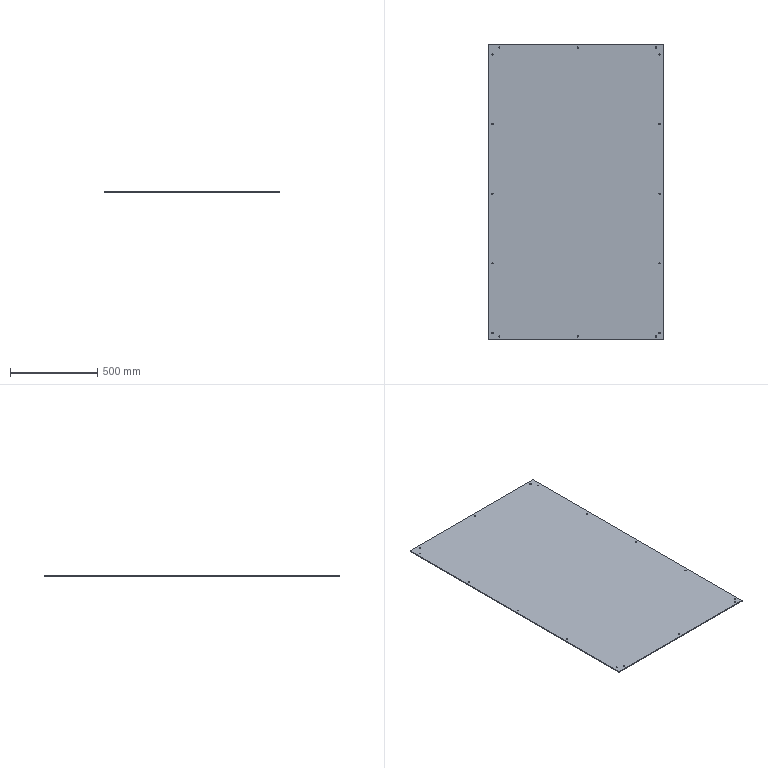Part | STEP file | 平铺封Plate_LE0314013532 | 1 solid | 42 faces | box 1000 x 1700 x 5 mm | volume 8497328 mm3 | cylinder 36 | plane 6 | commonest cylinder face diameters 6.5 x32 4 x4
STEP:
#1=CARTESIAN_POINT('',(463.25,-830.,-2.5));
#2=VERTEX_POINT('',#1);
#3=CARTESIAN_POINT('',(456.75,-830.,-2.5));
#4=VERTEX_POINT('',#3);
#5=CARTESIAN_POINT('',(460.,-830.,-2.5));
#6=DIRECTION('',(0.,0.,-1.));
#7=DIRECTION('',(1.,0.,0.));
#8=AXIS2_PLACEMENT_3D('',#5,#6,#7);
#9=CIRCLE('',#8,3.25);
#10=EDGE_CURVE('',#2,#4,#9,.T.);
#11=ORIENTED_EDGE('',*,*,#10,.T.);
#12=CARTESIAN_POINT('',(456.75,-830.,2.5));
#13=VERTEX_POINT('',#12);
#14=CARTESIAN_POINT('',(456.75,-830.,2.5));
#15=DIRECTION('',(0.,0.,1.));
#16=VECTOR('',#15,1000.);
#17=LINE('',#14,#16);
#18=EDGE_CURVE('',#4,#13,#17,.T.);
#19=ORIENTED_EDGE('',*,*,#18,.T.);
#20=CARTESIAN_POINT('',(463.25,-830.,2.5));
#21=VERTEX_POINT('',#20);
#22=CARTESIAN_POINT('',(460.,-830.,2.5));
#23=DIRECTION('',(0.,0.,-1.));
#24=DIRECTION('',(1.,0.,0.));
#25=AXIS2_PLACEMENT_3D('',#22,#23,#24);
#26=CIRCLE('',#25,3.25);
#27=EDGE_CURVE('',#21,#13,#26,.T.);
#28=ORIENTED_EDGE('',*,*,#27,.F.);
#29=CARTESIAN_POINT('',(463.25,-830.,2.5));
#30=DIRECTION('',(0.,0.,1.));
#31=VECTOR('',#30,1000.);
#32=LINE('',#29,#31);
#33=EDGE_CURVE('',#2,#21,#32,.T.);
#34=ORIENTED_EDGE('',*,*,#33,.F.);
#35=EDGE_LOOP('',(#11,#19,#28,#34));
#36=FACE_OUTER_BOUND('',#35,.T.);
#37=CARTESIAN_POINT('',(460.,-830.,2.5));
#38=DIRECTION('',(0.,0.,1.));
#39=DIRECTION('',(1.,0.,0.));
#40=AXIS2_PLACEMENT_3D('',#37,#38,#39);
#41=CYLINDRICAL_SURFACE('',#40,3.25);
#42=ADVANCED_FACE('',(#36),#41,.F.);
#43=CARTESIAN_POINT('',(463.25,830.,-2.5));
#44=VERTEX_POINT('',#43);
#45=CARTESIAN_POINT('',(456.75,830.,-2.5));
#46=VERTEX_POINT('',#45);
#47=CARTESIAN_POINT('',(460.,830.,-2.5));
#48=DIRECTION('',(0.,0.,-1.));
#49=DIRECTION('',(1.,0.,0.));
#50=AXIS2_PLACEMENT_3D('',#47,#48,#49);
#51=CIRCLE('',#50,3.25);
#52=EDGE_CURVE('',#44,#46,#51,.T.);
#53=ORIENTED_EDGE('',*,*,#52,.T.);
#54=CARTESIAN_POINT('',(456.75,830.,2.5));
#55=VERTEX_POINT('',#54);
#56=CARTESIAN_POINT('',(456.75,830.,2.5));
#57=DIRECTION('',(0.,0.,1.));
#58=VECTOR('',#57,1000.);
#59=LINE('',#56,#58);
#60=EDGE_CURVE('',#46,#55,#59,.T.);
#61=ORIENTED_EDGE('',*,*,#60,.T.);
#62=CARTESIAN_POINT('',(463.25,830.,2.5));
#63=VERTEX_POINT('',#62);
#64=CARTESIAN_POINT('',(460.,830.,2.5));
#65=DIRECTION('',(0.,0.,-1.));
#66=DIRECTION('',(1.,0.,0.));
#67=AXIS2_PLACEMENT_3D('',#64,#65,#66);
#68=CIRCLE('',#67,3.25);
#69=EDGE_CURVE('',#63,#55,#68,.T.);
#70=ORIENTED_EDGE('',*,*,#69,.F.);
#71=CARTESIAN_POINT('',(463.25,830.,2.5));
#72=DIRECTION('',(0.,0.,1.));
#73=VECTOR('',#72,1000.);
#74=LINE('',#71,#73);
#75=EDGE_CURVE('',#44,#63,#74,.T.);
#76=ORIENTED_EDGE('',*,*,#75,.F.);
#77=EDGE_LOOP('',(#53,#61,#70,#76));
#78=FACE_OUTER_BOUND('',#77,.T.);
#79=CARTESIAN_POINT('',(460.,830.,2.5));
#80=DIRECTION('',(0.,0.,1.));
#81=DIRECTION('',(1.,0.,0.));
#82=AXIS2_PLACEMENT_3D('',#79,#80,#81);
#83=CYLINDRICAL_SURFACE('',#82,3.25);
#84=ADVANCED_FACE('',(#78),#83,.F.);
#85=CARTESIAN_POINT('',(-476.75,-810.,-2.5));
#86=VERTEX_POINT('',#85);
#87=CARTESIAN_POINT('',(-483.25,-810.,-2.5));
#88=VERTEX_POINT('',#87);
#89=CARTESIAN_POINT('',(-480.,-810.,-2.5));
#90=DIRECTION('',(0.,0.,-1.));
#91=DIRECTION('',(1.,0.,0.));
#92=AXIS2_PLACEMENT_3D('',#89,#90,#91);
#93=CIRCLE('',#92,3.25);
#94=EDGE_CURVE('',#86,#88,#93,.T.);
#95=ORIENTED_EDGE('',*,*,#94,.T.);
#96=CARTESIAN_POINT('',(-483.25,-810.,2.5));
#97=VERTEX_POINT('',#96);
#98=CARTESIAN_POINT('',(-483.25,-810.,2.5));
#99=DIRECTION('',(0.,0.,1.));
#100=VECTOR('',#99,1000.);
#101=LINE('',#98,#100);
#102=EDGE_CURVE('',#88,#97,#101,.T.);
#103=ORIENTED_EDGE('',*,*,#102,.T.);
#104=CARTESIAN_POINT('',(-476.75,-810.,2.5));
#105=VERTEX_POINT('',#104);
#106=CARTESIAN_POINT('',(-480.,-810.,2.5));
#107=DIRECTION('',(0.,0.,-1.));
#108=DIRECTION('',(1.,0.,0.));
#109=AXIS2_PLACEMENT_3D('',#106,#107,#108);
#110=CIRCLE('',#109,3.25);
#111=EDGE_CURVE('',#105,#97,#110,.T.);
#112=ORIENTED_EDGE('',*,*,#111,.F.);
#113=CARTESIAN_POINT('',(-476.75,-810.,2.5));
#114=DIRECTION('',(0.,0.,1.));
#115=VECTOR('',#114,1000.);
#116=LINE('',#113,#115);
#117=EDGE_CURVE('',#86,#105,#116,.T.);
#118=ORIENTED_EDGE('',*,*,#117,.F.);
#119=EDGE_LOOP('',(#95,#103,#112,#118));
#120=FACE_OUTER_BOUND('',#119,.T.);
#121=CARTESIAN_POINT('',(-480.,-810.,2.5));
#122=DIRECTION('',(0.,0.,1.));
#123=DIRECTION('',(1.,0.,0.));
#124=AXIS2_PLACEMENT_3D('',#121,#122,#123);
#125=CYLINDRICAL_SURFACE('',#124,3.25);
#126=ADVANCED_FACE('',(#120),#125,.F.);
#127=CARTESIAN_POINT('',(-476.75,-410.,-2.5));
#128=VERTEX_POINT('',#127);
#129=CARTESIAN_POINT('',(-483.25,-410.,-2.5));
#130=VERTEX_POINT('',#129);
#131=CARTESIAN_POINT('',(-480.,-410.,-2.5));
#132=DIRECTION('',(0.,0.,-1.));
#133=DIRECTION('',(1.,0.,0.));
#134=AXIS2_PLACEMENT_3D('',#131,#132,#133);
#135=CIRCLE('',#134,3.25);
#136=EDGE_CURVE('',#128,#130,#135,.T.);
#137=ORIENTED_EDGE('',*,*,#136,.T.);
#138=CARTESIAN_POINT('',(-483.25,-410.,2.5));
#139=VERTEX_POINT('',#138);
#140=CARTESIAN_POINT('',(-483.25,-410.,2.5));
#141=DIRECTION('',(0.,0.,1.));
#142=VECTOR('',#141,1000.);
#143=LINE('',#140,#142);
#144=EDGE_CURVE('',#130,#139,#143,.T.);
#145=ORIENTED_EDGE('',*,*,#144,.T.);
#146=CARTESIAN_POINT('',(-476.75,-410.,2.5));
#147=VERTEX_POINT('',#146);
#148=CARTESIAN_POINT('',(-480.,-410.,2.5));
#149=DIRECTION('',(0.,0.,-1.));
#150=DIRECTION('',(1.,0.,0.));
#151=AXIS2_PLACEMENT_3D('',#148,#149,#150);
#152=CIRCLE('',#151,3.25);
#153=EDGE_CURVE('',#147,#139,#152,.T.);
#154=ORIENTED_EDGE('',*,*,#153,.F.);
#155=CARTESIAN_POINT('',(-476.75,-410.,2.5));
#156=DIRECTION('',(0.,0.,1.));
#157=VECTOR('',#156,1000.);
#158=LINE('',#155,#157);
#159=EDGE_CURVE('',#128,#147,#158,.T.);
#160=ORIENTED_EDGE('',*,*,#159,.F.);
#161=EDGE_LOOP('',(#137,#145,#154,#160));
#162=FACE_OUTER_BOUND('',#161,.T.);
#163=CARTESIAN_POINT('',(-480.,-410.,2.5));
#164=DIRECTION('',(0.,0.,1.));
#165=DIRECTION('',(1.,0.,0.));
#166=AXIS2_PLACEMENT_3D('',#163,#164,#165);
#167=CYLINDRICAL_SURFACE('',#166,3.25);
#168=ADVANCED_FACE('',(#162),#167,.F.);
#169=CARTESIAN_POINT('',(-476.75,-10.,-2.5));
#170=VERTEX_POINT('',#169);
#171=CARTESIAN_POINT('',(-483.25,-10.,-2.5));
#172=VERTEX_POINT('',#171);
#173=CARTESIAN_POINT('',(-480.,-10.,-2.5));
#174=DIRECTION('',(0.,0.,-1.));
#175=DIRECTION('',(1.,0.,0.));
#176=AXIS2_PLACEMENT_3D('',#173,#174,#175);
#177=CIRCLE('',#176,3.25);
#178=EDGE_CURVE('',#170,#172,#177,.T.);
#179=ORIENTED_EDGE('',*,*,#178,.T.);
#180=CARTESIAN_POINT('',(-483.25,-10.,2.5));
#181=VERTEX_POINT('',#180);
#182=CARTESIAN_POINT('',(-483.25,-10.,2.5));
#183=DIRECTION('',(0.,0.,1.));
#184=VECTOR('',#183,1000.);
#185=LINE('',#182,#184);
#186=EDGE_CURVE('',#172,#181,#185,.T.);
#187=ORIENTED_EDGE('',*,*,#186,.T.);
#188=CARTESIAN_POINT('',(-476.75,-10.,2.5));
#189=VERTEX_POINT('',#188);
#190=CARTESIAN_POINT('',(-480.,-10.,2.5));
#191=DIRECTION('',(0.,0.,-1.));
#192=DIRECTION('',(1.,0.,0.));
#193=AXIS2_PLACEMENT_3D('',#190,#191,#192);
#194=CIRCLE('',#193,3.25);
#195=EDGE_CURVE('',#189,#181,#194,.T.);
#196=ORIENTED_EDGE('',*,*,#195,.F.);
#197=CARTESIAN_POINT('',(-476.75,-10.,2.5));
#198=DIRECTION('',(0.,0.,1.));
#199=VECTOR('',#198,1000.);
#200=LINE('',#197,#199);
#201=EDGE_CURVE('',#170,#189,#200,.T.);
#202=ORIENTED_EDGE('',*,*,#201,.F.);
#203=EDGE_LOOP('',(#179,#187,#196,#202));
#204=FACE_OUTER_BOUND('',#203,.T.);
#205=CARTESIAN_POINT('',(-480.,-10.,2.5));
#206=DIRECTION('',(0.,0.,1.));
#207=DIRECTION('',(1.,0.,0.));
#208=AXIS2_PLACEMENT_3D('',#205,#206,#207);
#209=CYLINDRICAL_SURFACE('',#208,3.25);
#210=ADVANCED_FACE('',(#204),#209,.F.);
#211=CARTESIAN_POINT('',(483.25,-810.,-2.5));
#212=VERTEX_POINT('',#211);
#213=CARTESIAN_POINT('',(476.75,-810.,-2.5));
#214=VERTEX_POINT('',#213);
#215=CARTESIAN_POINT('',(480.,-810.,-2.5));
#216=DIRECTION('',(0.,0.,-1.));
#217=DIRECTION('',(1.,0.,0.));
#218=AXIS2_PLACEMENT_3D('',#215,#216,#217);
#219=CIRCLE('',#218,3.25);
#220=EDGE_CURVE('',#212,#214,#219,.T.);
#221=ORIENTED_EDGE('',*,*,#220,.T.);
#222=CARTESIAN_POINT('',(476.75,-810.,2.5));
#223=VERTEX_POINT('',#222);
#224=CARTESIAN_POINT('',(476.75,-810.,2.5));
#225=DIRECTION('',(0.,0.,1.));
#226=VECTOR('',#225,1000.);
#227=LINE('',#224,#226);
#228=EDGE_CURVE('',#214,#223,#227,.T.);
#229=ORIENTED_EDGE('',*,*,#228,.T.);
#230=CARTESIAN_POINT('',(483.25,-810.,2.5));
#231=VERTEX_POINT('',#230);
#232=CARTESIAN_POINT('',(480.,-810.,2.5));
#233=DIRECTION('',(0.,0.,-1.));
#234=DIRECTION('',(1.,0.,0.));
#235=AXIS2_PLACEMENT_3D('',#232,#233,#234);
#236=CIRCLE('',#235,3.25);
#237=EDGE_CURVE('',#231,#223,#236,.T.);
#238=ORIENTED_EDGE('',*,*,#237,.F.);
#239=CARTESIAN_POINT('',(483.25,-810.,2.5));
#240=DIRECTION('',(0.,0.,1.));
#241=VECTOR('',#240,1000.);
#242=LINE('',#239,#241);
#243=EDGE_CURVE('',#212,#231,#242,.T.);
#244=ORIENTED_EDGE('',*,*,#243,.F.);
#245=EDGE_LOOP('',(#221,#229,#238,#244));
#246=FACE_OUTER_BOUND('',#245,.T.);
#247=CARTESIAN_POINT('',(480.,-810.,2.5));
#248=DIRECTION('',(0.,0.,1.));
#249=DIRECTION('',(1.,0.,0.));
#250=AXIS2_PLACEMENT_3D('',#247,#248,#249);
#251=CYLINDRICAL_SURFACE('',#250,3.25);
#252=ADVANCED_FACE('',(#246),#251,.F.);
#253=CARTESIAN_POINT('',(483.25,-410.,-2.5));
#254=VERTEX_POINT('',#253);
#255=CARTESIAN_POINT('',(476.75,-410.,-2.5));
#256=VERTEX_POINT('',#255);
#257=CARTESIAN_POINT('',(480.,-410.,-2.5));
#258=DIRECTION('',(0.,0.,-1.));
#259=DIRECTION('',(1.,0.,0.));
#260=AXIS2_PLACEMENT_3D('',#257,#258,#259);
#261=CIRCLE('',#260,3.25);
#262=EDGE_CURVE('',#254,#256,#261,.T.);
#263=ORIENTED_EDGE('',*,*,#262,.T.);
#264=CARTESIAN_POINT('',(476.75,-410.,2.5));
#265=VERTEX_POINT('',#264);
#266=CARTESIAN_POINT('',(476.75,-410.,2.5));
#267=DIRECTION('',(0.,0.,1.));
#268=VECTOR('',#267,1000.);
#269=LINE('',#266,#268);
#270=EDGE_CURVE('',#256,#265,#269,.T.);
#271=ORIENTED_EDGE('',*,*,#270,.T.);
#272=CARTESIAN_POINT('',(483.25,-410.,2.5));
#273=VERTEX_POINT('',#272);
#274=CARTESIAN_POINT('',(480.,-410.,2.5));
#275=DIRECTION('',(0.,0.,-1.));
#276=DIRECTION('',(1.,0.,0.));
#277=AXIS2_PLACEMENT_3D('',#274,#275,#276);
#278=CIRCLE('',#277,3.25);
#279=EDGE_CURVE('',#273,#265,#278,.T.);
#280=ORIENTED_EDGE('',*,*,#279,.F.);
#281=CARTESIAN_POINT('',(483.25,-410.,2.5));
#282=DIRECTION('',(0.,0.,1.));
#283=VECTOR('',#282,1000.);
#284=LINE('',#281,#283);
#285=EDGE_CURVE('',#254,#273,#284,.T.);
#286=ORIENTED_EDGE('',*,*,#285,.F.);
#287=EDGE_LOOP('',(#263,#271,#280,#286));
#288=FACE_OUTER_BOUND('',#287,.T.);
#289=CARTESIAN_POINT('',(480.,-410.,2.5));
#290=DIRECTION('',(0.,0.,1.));
#291=DIRECTION('',(1.,0.,0.));
#292=AXIS2_PLACEMENT_3D('',#289,#290,#291);
#293=CYLINDRICAL_SURFACE('',#292,3.25);
#294=ADVANCED_FACE('',(#288),#293,.F.);
#295=CARTESIAN_POINT('',(483.25,-10.,-2.5));
#296=VERTEX_POINT('',#295);
#297=CARTESIAN_POINT('',(476.75,-10.,-2.5));
#298=VERTEX_POINT('',#297);
#299=CARTESIAN_POINT('',(480.,-10.,-2.5));
#300=DIRECTION('',(0.,0.,-1.));
#301=DIRECTION('',(1.,0.,0.));
#302=AXIS2_PLACEMENT_3D('',#299,#300,#301);
#303=CIRCLE('',#302,3.25);
#304=EDGE_CURVE('',#296,#298,#303,.T.);
#305=ORIENTED_EDGE('',*,*,#304,.T.);
#306=CARTESIAN_POINT('',(476.75,-10.,2.5));
#307=VERTEX_POINT('',#306);
#308=CARTESIAN_POINT('',(476.75,-10.,2.5));
#309=DIRECTION('',(0.,0.,1.));
#310=VECTOR('',#309,1000.);
#311=LINE('',#308,#310);
#312=EDGE_CURVE('',#298,#307,#311,.T.);
#313=ORIENTED_EDGE('',*,*,#312,.T.);
#314=CARTESIAN_POINT('',(483.25,-10.,2.5));
#315=VERTEX_POINT('',#314);
#316=CARTESIAN_POINT('',(480.,-10.,2.5));
#317=DIRECTION('',(0.,0.,-1.));
#318=DIRECTION('',(1.,0.,0.));
#319=AXIS2_PLACEMENT_3D('',#316,#317,#318);
#320=CIRCLE('',#319,3.25);
#321=EDGE_CURVE('',#315,#307,#320,.T.);
#322=ORIENTED_EDGE('',*,*,#321,.F.);
#323=CARTESIAN_POINT('',(483.25,-10.,2.5));
#324=DIRECTION('',(0.,0.,1.));
#325=VECTOR('',#324,1000.);
#326=LINE('',#323,#325);
#327=EDGE_CURVE('',#296,#315,#326,.T.);
#328=ORIENTED_EDGE('',*,*,#327,.F.);
#329=EDGE_LOOP('',(#305,#313,#322,#328));
#330=FACE_OUTER_BOUND('',#329,.T.);
#331=CARTESIAN_POINT('',(480.,-10.,2.5));
#332=DIRECTION('',(0.,0.,1.));
#333=DIRECTION('',(1.,0.,0.));
#334=AXIS2_PLACEMENT_3D('',#331,#332,#333);
#335=CYLINDRICAL_SURFACE('',#334,3.25);
#336=ADVANCED_FACE('',(#330),#335,.F.);
#337=CARTESIAN_POINT('',(-476.75,790.,-2.5));
#338=VERTEX_POINT('',#337);
#339=CARTESIAN_POINT('',(-483.25,790.,-2.5));
#340=VERTEX_POINT('',#339);
#341=CARTESIAN_POINT('',(-480.,790.,-2.5));
#342=DIRECTION('',(0.,0.,-1.));
#343=DIRECTION('',(1.,0.,0.));
#344=AXIS2_PLACEMENT_3D('',#341,#342,#343);
#345=CIRCLE('',#344,3.25);
#346=EDGE_CURVE('',#338,#340,#345,.T.);
#347=ORIENTED_EDGE('',*,*,#346,.T.);
#348=CARTESIAN_POINT('',(-483.25,790.,2.5));
#349=VERTEX_POINT('',#348);
#350=CARTESIAN_POINT('',(-483.25,790.,2.5));
#351=DIRECTION('',(0.,0.,1.));
#352=VECTOR('',#351,1000.);
#353=LINE('',#350,#352);
#354=EDGE_CURVE('',#340,#349,#353,.T.);
#355=ORIENTED_EDGE('',*,*,#354,.T.);
#356=CARTESIAN_POINT('',(-476.75,790.,2.5));
#357=VERTEX_POINT('',#356);
#358=CARTESIAN_POINT('',(-480.,790.,2.5));
#359=DIRECTION('',(0.,0.,-1.));
#360=DIRECTION('',(1.,0.,0.));
#361=AXIS2_PLACEMENT_3D('',#358,#359,#360);
#362=CIRCLE('',#361,3.25);
#363=EDGE_CURVE('',#357,#349,#362,.T.);
#364=ORIENTED_EDGE('',*,*,#363,.F.);
#365=CARTESIAN_POINT('',(-476.75,790.,2.5));
#366=DIRECTION('',(0.,0.,1.));
#367=VECTOR('',#366,1000.);
#368=LINE('',#365,#367);
#369=EDGE_CURVE('',#338,#357,#368,.T.);
#370=ORIENTED_EDGE('',*,*,#369,.F.);
#371=EDGE_LOOP('',(#347,#355,#364,#370));
#372=FACE_OUTER_BOUND('',#371,.T.);
#373=CARTESIAN_POINT('',(-480.,790.,2.5));
#374=DIRECTION('',(0.,0.,1.));
#375=DIRECTION('',(1.,0.,0.));
#376=AXIS2_PLACEMENT_3D('',#373,#374,#375);
#377=CYLINDRICAL_SURFACE('',#376,3.25);
#378=ADVANCED_FACE('',(#372),#377,.F.);
#379=CARTESIAN_POINT('',(-436.75,-830.,-2.5));
#380=VERTEX_POINT('',#379);
#381=CARTESIAN_POINT('',(-443.25,-830.,-2.5));
#382=VERTEX_POINT('',#381);
#383=CARTESIAN_POINT('',(-440.,-830.,-2.5));
#384=DIRECTION('',(0.,0.,-1.));
#385=DIRECTION('',(1.,0.,0.));
#386=AXIS2_PLACEMENT_3D('',#383,#384,#385);
#387=CIRCLE('',#386,3.25);
#388=EDGE_CURVE('',#380,#382,#387,.T.);
#389=ORIENTED_EDGE('',*,*,#388,.T.);
#390=CARTESIAN_POINT('',(-443.25,-830.,2.5));
#391=VERTEX_POINT('',#390);
#392=CARTESIAN_POINT('',(-443.25,-830.,2.5));
#393=DIRECTION('',(0.,0.,1.));
#394=VECTOR('',#393,1000.);
#395=LINE('',#392,#394);
#396=EDGE_CURVE('',#382,#391,#395,.T.);
#397=ORIENTED_EDGE('',*,*,#396,.T.);
#398=CARTESIAN_POINT('',(-436.75,-830.,2.5));
#399=VERTEX_POINT('',#398);
#400=CARTESIAN_POINT('',(-440.,-830.,2.5));
#401=DIRECTION('',(0.,0.,-1.));
#402=DIRECTION('',(1.,0.,0.));
#403=AXIS2_PLACEMENT_3D('',#400,#401,#402);
#404=CIRCLE('',#403,3.25);
#405=EDGE_CURVE('',#399,#391,#404,.T.);
#406=ORIENTED_EDGE('',*,*,#405,.F.);
#407=CARTESIAN_POINT('',(-436.75,-830.,2.5));
#408=DIRECTION('',(0.,0.,1.));
#409=VECTOR('',#408,1000.);
#410=LINE('',#407,#409);
#411=EDGE_CURVE('',#380,#399,#410,.T.);
#412=ORIENTED_EDGE('',*,*,#411,.F.);
#413=EDGE_LOOP('',(#389,#397,#406,#412));
#414=FACE_OUTER_BOUND('',#413,.T.);
#415=CARTESIAN_POINT('',(-440.,-830.,2.5));
#416=DIRECTION('',(0.,0.,1.));
#417=DIRECTION('',(1.,0.,0.));
#418=AXIS2_PLACEMENT_3D('',#415,#416,#417);
#419=CYLINDRICAL_SURFACE('',#418,3.25);
#420=ADVANCED_FACE('',(#414),#419,.F.);
#421=CARTESIAN_POINT('',(483.25,790.,-2.5));
#422=VERTEX_POINT('',#421);
#423=CARTESIAN_POINT('',(476.75,790.,-2.5));
#424=VERTEX_POINT('',#423);
#425=CARTESIAN_POINT('',(480.,790.,-2.5));
#426=DIRECTION('',(0.,0.,-1.));
#427=DIRECTION('',(1.,0.,0.));
#428=AXIS2_PLACEMENT_3D('',#425,#426,#427);
#429=CIRCLE('',#428,3.25);
#430=EDGE_CURVE('',#422,#424,#429,.T.);
#431=ORIENTED_EDGE('',*,*,#430,.T.);
#432=CARTESIAN_POINT('',(476.75,790.,2.5));
#433=VERTEX_POINT('',#432);
#434=CARTESIAN_POINT('',(476.75,790.,2.5));
#435=DIRECTION('',(0.,0.,1.));
#436=VECTOR('',#435,1000.);
#437=LINE('',#434,#436);
#438=EDGE_CURVE('',#424,#433,#437,.T.);
#439=ORIENTED_EDGE('',*,*,#438,.T.);
#440=CARTESIAN_POINT('',(483.25,790.,2.5));
#441=VERTEX_POINT('',#440);
#442=CARTESIAN_POINT('',(480.,790.,2.5));
#443=DIRECTION('',(0.,0.,-1.));
#444=DIRECTION('',(1.,0.,0.));
#445=AXIS2_PLACEMENT_3D('',#442,#443,#444);
#446=CIRCLE('',#445,3.25);
#447=EDGE_CURVE('',#441,#433,#446,.T.);
#448=ORIENTED_EDGE('',*,*,#447,.F.);
#449=CARTESIAN_POINT('',(483.25,790.,2.5));
#450=DIRECTION('',(0.,0.,1.));
#451=VECTOR('',#450,1000.);
#452=LINE('',#449,#451);
#453=EDGE_CURVE('',#422,#441,#452,.T.);
#454=ORIENTED_EDGE('',*,*,#453,.F.);
#455=EDGE_LOOP('',(#431,#439,#448,#454));
#456=FACE_OUTER_BOUND('',#455,.T.);
#457=CARTESIAN_POINT('',(480.,790.,2.5));
#458=DIRECTION('',(0.,0.,1.));
#459=DIRECTION('',(1.,0.,0.));
#460=AXIS2_PLACEMENT_3D('',#457,#458,#459);
#461=CYLINDRICAL_SURFACE('',#460,3.25);
#462=ADVANCED_FACE('',(#456),#461,.F.);
#463=CARTESIAN_POINT('',(-436.75,830.,-2.5));
#464=VERTEX_POINT('',#463);
#465=CARTESIAN_POINT('',(-443.25,830.,-2.5));
#466=VERTEX_POINT('',#465);
#467=CARTESIAN_POINT('',(-440.,830.,-2.5));
#468=DIRECTION('',(0.,0.,-1.));
#469=DIRECTION('',(1.,0.,0.));
#470=AXIS2_PLACEMENT_3D('',#467,#468,#469);
#471=CIRCLE('',#470,3.25);
#472=EDGE_CURVE('',#464,#466,#471,.T.);
#473=ORIENTED_EDGE('',*,*,#472,.T.);
#474=CARTESIAN_POINT('',(-443.25,830.,2.5));
#475=VERTEX_POINT('',#474);
#476=CARTESIAN_POINT('',(-443.25,830.,2.5));
#477=DIRECTION('',(0.,0.,1.));
#478=VECTOR('',#477,1000.);
#479=LINE('',#476,#478);
#480=EDGE_CURVE('',#466,#475,#479,.T.);
#481=ORIENTED_EDGE('',*,*,#480,.T.);
#482=CARTESIAN_POINT('',(-436.75,830.,2.5));
#483=VERTEX_POINT('',#482);
#484=CARTESIAN_POINT('',(-440.,830.,2.5));
#485=DIRECTION('',(0.,0.,-1.));
#486=DIRECTION('',(1.,0.,0.));
#487=AXIS2_PLACEMENT_3D('',#484,#485,#486);
#488=CIRCLE('',#487,3.25);
#489=EDGE_CURVE('',#483,#475,#488,.T.);
#490=ORIENTED_EDGE('',*,*,#489,.F.);
#491=CARTESIAN_POINT('',(-436.75,830.,2.5));
#492=DIRECTION('',(0.,0.,1.));
#493=VECTOR('',#492,1000.);
#494=LINE('',#491,#493);
#495=EDGE_CURVE('',#464,#483,#494,.T.);
#496=ORIENTED_EDGE('',*,*,#495,.F.);
#497=EDGE_LOOP('',(#473,#481,#490,#496));
#498=FACE_OUTER_BOUND('',#497,.T.);
#499=CARTESIAN_POINT('',(-440.,830.,2.5));
#500=DIRECTION('',(0.,0.,1.));
#501=DIRECTION('',(1.,0.,0.));
#502=AXIS2_PLACEMENT_3D('',#499,#500,#501);
#503=CYLINDRICAL_SURFACE('',#502,3.25);
#504=ADVANCED_FACE('',(#498),#503,.F.);
#505=CARTESIAN_POINT('',(483.25,390.,-2.5));
#506=VERTEX_POINT('',#505);
#507=CARTESIAN_POINT('',(476.75,390.,-2.5));
#508=VERTEX_POINT('',#507);
#509=CARTESIAN_POINT('',(480.,390.,-2.5));
#510=DIRECTION('',(0.,0.,-1.));
#511=DIRECTION('',(1.,0.,0.));
#512=AXIS2_PLACEMENT_3D('',#509,#510,#511);
#513=CIRCLE('',#512,3.25);
#514=EDGE_CURVE('',#506,#508,#513,.T.);
#515=ORIENTED_EDGE('',*,*,#514,.T.);
#516=CARTESIAN_POINT('',(476.75,390.,2.5));
#517=VERTEX_POINT('',#516);
#518=CARTESIAN_POINT('',(476.75,390.,2.5));
#519=DIRECTION('',(0.,0.,1.));
#520=VECTOR('',#519,1000.);
#521=LINE('',#518,#520);
#522=EDGE_CURVE('',#508,#517,#521,.T.);
#523=ORIENTED_EDGE('',*,*,#522,.T.);
#524=CARTESIAN_POINT('',(483.25,390.,2.5));
#525=VERTEX_POINT('',#524);
#526=CARTESIAN_POINT('',(480.,390.,2.5));
#527=DIRECTION('',(0.,0.,-1.));
#528=DIRECTION('',(1.,0.,0.));
#529=AXIS2_PLACEMENT_3D('',#526,#527,#528);
#530=CIRCLE('',#529,3.25);
#531=EDGE_CURVE('',#525,#517,#530,.T.);
#532=ORIENTED_EDGE('',*,*,#531,.F.);
#533=CARTESIAN_POINT('',(483.25,390.,2.5));
#534=DIRECTION('',(0.,0.,1.));
#535=VECTOR('',#534,1000.);
#536=LINE('',#533,#535);
#537=EDGE_CURVE('',#506,#525,#536,.T.);
#538=ORIENTED_EDGE('',*,*,#537,.F.);
#539=EDGE_LOOP('',(#515,#523,#532,#538));
#540=FACE_OUTER_BOUND('',#539,.T.);
#541=CARTESIAN_POINT('',(480.,390.,2.5));
#542=DIRECTION('',(0.,0.,1.));
#543=DIRECTION('',(1.,0.,0.));
#544=AXIS2_PLACEMENT_3D('',#541,#542,#543);
#545=CYLINDRICAL_SURFACE('',#544,3.25);
#546=ADVANCED_FACE('',(#540),#545,.F.);
#547=CARTESIAN_POINT('',(-476.75,390.,-2.5));
#548=VERTEX_POINT('',#547);
#549=CARTESIAN_POINT('',(-483.25,390.,-2.5));
#550=VERTEX_POINT('',#549);
#551=CARTESIAN_POINT('',(-480.,390.,-2.5));
#552=DIRECTION('',(0.,0.,-1.));
#553=DIRECTION('',(1.,0.,0.));
#554=AXIS2_PLACEMENT_3D('',#551,#552,#553);
#555=CIRCLE('',#554,3.25);
#556=EDGE_CURVE('',#548,#550,#555,.T.);
#557=ORIENTED_EDGE('',*,*,#556,.T.);
#558=CARTESIAN_POINT('',(-483.25,390.,2.5));
#559=VERTEX_POINT('',#558);
#560=CARTESIAN_POINT('',(-483.25,390.,2.5));
#561=DIRECTION('',(0.,0.,1.));
#562=VECTOR('',#561,1000.);
#563=LINE('',#560,#562);
#564=EDGE_CURVE('',#550,#559,#563,.T.);
#565=ORIENTED_EDGE('',*,*,#564,.T.);
#566=CARTESIAN_POINT('',(-476.75,390.,2.5));
#567=VERTEX_POINT('',#566);
#568=CARTESIAN_POINT('',(-480.,390.,2.5));
#569=DIRECTION('',(0.,0.,-1.));
#570=DIRECTION('',(1.,0.,0.));
#571=AXIS2_PLACEMENT_3D('',#568,#569,#570);
#572=CIRCLE('',#571,3.25);
#573=EDGE_CURVE('',#567,#559,#572,.T.);
#574=ORIENTED_EDGE('',*,*,#573,.F.);
#575=CARTESIAN_POINT('',(-476.75,390.,2.5));
#576=DIRECTION('',(0.,0.,1.));
#577=VECTOR('',#576,1000.);
#578=LINE('',#575,#577);
#579=EDGE_CURVE('',#548,#567,#578,.T.);
#580=ORIENTED_EDGE('',*,*,#579,.F.);
#581=EDGE_LOOP('',(#557,#565,#574,#580));
#582=FACE_OUTER_BOUND('',#581,.T.);
#583=CARTESIAN_POINT('',(-480.,390.,2.5));
#584=DIRECTION('',(0.,0.,1.));
#585=DIRECTION('',(1.,0.,0.));
#586=AXIS2_PLACEMENT_3D('',#583,#584,#585);
#587=CYLINDRICAL_SURFACE('',#586,3.25);
#588=ADVANCED_FACE('',(#582),#587,.F.);
#589=CARTESIAN_POINT('',(13.25,830.,-2.5));
#590=VERTEX_POINT('',#589);
#591=CARTESIAN_POINT('',(6.75,830.,-2.5));
#592=VERTEX_POINT('',#591);
#593=CARTESIAN_POINT('',(10.,830.,-2.5));
#594=DIRECTION('',(0.,0.,-1.));
#595=DIRECTION('',(1.,0.,0.));
#596=AXIS2_PLACEMENT_3D('',#593,#594,#595);
#597=CIRCLE('',#596,3.25);
#598=EDGE_CURVE('',#590,#592,#597,.T.);
#599=ORIENTED_EDGE('',*,*,#598,.T.);
#600=CARTESIAN_POINT('',(6.75,830.,2.5));
#601=VERTEX_POINT('',#600);
#602=CARTESIAN_POINT('',(6.75,830.,2.5));
#603=DIRECTION('',(0.,0.,1.));
#604=VECTOR('',#603,1000.);
#605=LINE('',#602,#604);
#606=EDGE_CURVE('',#592,#601,#605,.T.);
#607=ORIENTED_EDGE('',*,*,#606,.T.);
#608=CARTESIAN_POINT('',(13.25,830.,2.5));
#609=VERTEX_POINT('',#608);
#610=CARTESIAN_POINT('',(10.,830.,2.5));
#611=DIRECTION('',(0.,0.,-1.));
#612=DIRECTION('',(1.,0.,0.));
#613=AXIS2_PLACEMENT_3D('',#610,#611,#612);
#614=CIRCLE('',#613,3.25);
#615=EDGE_CURVE('',#609,#601,#614,.T.);
#616=ORIENTED_EDGE('',*,*,#615,.F.);
#617=CARTESIAN_POINT('',(13.25,830.,2.5));
#618=DIRECTION('',(0.,0.,1.));
#619=VECTOR('',#618,1000.);
#620=LINE('',#617,#619);
#621=EDGE_CURVE('',#590,#609,#620,.T.);
#622=ORIENTED_EDGE('',*,*,#621,.F.);
#623=EDGE_LOOP('',(#599,#607,#616,#622));
#624=FACE_OUTER_BOUND('',#623,.T.);
#625=CARTESIAN_POINT('',(10.,830.,2.5));
#626=DIRECTION('',(0.,0.,1.));
#627=DIRECTION('',(1.,0.,0.));
#628=AXIS2_PLACEMENT_3D('',#625,#626,#627);
#629=CYLINDRICAL_SURFACE('',#628,3.25);
#630=ADVANCED_FACE('',(#624),#629,.F.);
#631=CARTESIAN_POINT('',(13.25,-830.,-2.5));
#632=VERTEX_POINT('',#631);
#633=CARTESIAN_POINT('',(6.75,-830.,-2.5));
#634=VERTEX_POINT('',#633);
#635=CARTESIAN_POINT('',(10.,-830.,-2.5));
#636=DIRECTION('',(0.,0.,-1.));
#637=DIRECTION('',(1.,0.,0.));
#638=AXIS2_PLACEMENT_3D('',#635,#636,#637);
#639=CIRCLE('',#638,3.25);
#640=EDGE_CURVE('',#632,#634,#639,.T.);
#641=ORIENTED_EDGE('',*,*,#640,.T.);
#642=CARTESIAN_POINT('',(6.75,-830.,2.5));
#643=VERTEX_POINT('',#642);
#644=CARTESIAN_POINT('',(6.75,-830.,2.5));
#645=DIRECTION('',(0.,0.,1.));
#646=VECTOR('',#645,1000.);
#647=LINE('',#644,#646);
#648=EDGE_CURVE('',#634,#643,#647,.T.);
#649=ORIENTED_EDGE('',*,*,#648,.T.);
#650=CARTESIAN_POINT('',(13.25,-830.,2.5));
#651=VERTEX_POINT('',#650);
#652=CARTESIAN_POINT('',(10.,-830.,2.5));
#653=DIRECTION('',(0.,0.,-1.));
#654=DIRECTION('',(1.,0.,0.));
#655=AXIS2_PLACEMENT_3D('',#652,#653,#654);
#656=CIRCLE('',#655,3.25);
#657=EDGE_CURVE('',#651,#643,#656,.T.);
#658=ORIENTED_EDGE('',*,*,#657,.F.);
#659=CARTESIAN_POINT('',(13.25,-830.,2.5));
#660=DIRECTION('',(0.,0.,1.));
#661=VECTOR('',#660,1000.);
#662=LINE('',#659,#661);
#663=EDGE_CURVE('',#632,#651,#662,.T.);
#664=ORIENTED_EDGE('',*,*,#663,.F.);
#665=EDGE_LOOP('',(#641,#649,#658,#664));
#666=FACE_OUTER_BOUND('',#665,.T.);
#667=CARTESIAN_POINT('',(10.,-830.,2.5));
#668=DIRECTION('',(0.,0.,1.));
#669=DIRECTION('',(1.,0.,0.));
#670=AXIS2_PLACEMENT_3D('',#667,#668,#669);
#671=CYLINDRICAL_SURFACE('',#670,3.25);
#672=ADVANCED_FACE('',(#666),#671,.F.);
#673=ORIENTED_EDGE('',*,*,#10,.F.);
#674=CARTESIAN_POINT('',(460.,-830.,-2.5));
#675=DIRECTION('',(0.,0.,-1.));
#676=DIRECTION('',(1.,0.,0.));
#677=AXIS2_PLACEMENT_3D('',#674,#675,#676);
#678=CIRCLE('',#677,3.25);
#679=EDGE_CURVE('',#4,#2,#678,.T.);
#680=ORIENTED_EDGE('',*,*,#679,.F.);
#681=EDGE_LOOP('',(#673,#680));
#682=FACE_BOUND('',#681,.T.);
#683=ORIENTED_EDGE('',*,*,#52,.F.);
#684=CARTESIAN_POINT('',(460.,830.,-2.5));
#685=DIRECTION('',(0.,0.,-1.));
#686=DIRECTION('',(1.,0.,0.));
#687=AXIS2_PLACEMENT_3D('',#684,#685,#686);
#688=CIRCLE('',#687,3.25);
#689=EDGE_CURVE('',#46,#44,#688,.T.);
#690=ORIENTED_EDGE('',*,*,#689,.F.);
#691=EDGE_LOOP('',(#683,#690));
#692=FACE_BOUND('',#691,.T.);
#693=ORIENTED_EDGE('',*,*,#94,.F.);
#694=CARTESIAN_POINT('',(-480.,-810.,-2.5));
#695=DIRECTION('',(0.,0.,-1.));
#696=DIRECTION('',(1.,0.,0.));
#697=AXIS2_PLACEMENT_3D('',#694,#695,#696);
#698=CIRCLE('',#697,3.25);
#699=EDGE_CURVE('',#88,#86,#698,.T.);
#700=ORIENTED_EDGE('',*,*,#699,.F.);
#701=EDGE_LOOP('',(#693,#700));
#702=FACE_BOUND('',#701,.T.);
#703=ORIENTED_EDGE('',*,*,#136,.F.);
#704=CARTESIAN_POINT('',(-480.,-410.,-2.5));
#705=DIRECTION('',(0.,0.,-1.));
#706=DIRECTION('',(1.,0.,0.));
#707=AXIS2_PLACEMENT_3D('',#704,#705,#706);
#708=CIRCLE('',#707,3.25);
#709=EDGE_CURVE('',#130,#128,#708,.T.);
#710=ORIENTED_EDGE('',*,*,#709,.F.);
#711=EDGE_LOOP('',(#703,#710));
#712=FACE_BOUND('',#711,.T.);
#713=ORIENTED_EDGE('',*,*,#178,.F.);
#714=CARTESIAN_POINT('',(-480.,-10.,-2.5));
#715=DIRECTION('',(0.,0.,-1.));
#716=DIRECTION('',(1.,0.,0.));
#717=AXIS2_PLACEMENT_3D('',#714,#715,#716);
#718=CIRCLE('',#717,3.25);
#719=EDGE_CURVE('',#172,#170,#718,.T.);
#720=ORIENTED_EDGE('',*,*,#719,.F.);
#721=EDGE_LOOP('',(#713,#720));
#722=FACE_BOUND('',#721,.T.);
#723=ORIENTED_EDGE('',*,*,#220,.F.);
#724=CARTESIAN_POINT('',(480.,-810.,-2.5));
#725=DIRECTION('',(0.,0.,-1.));
#726=DIRECTION('',(1.,0.,0.));
#727=AXIS2_PLACEMENT_3D('',#724,#725,#726);
#728=CIRCLE('',#727,3.25);
#729=EDGE_CURVE('',#214,#212,#728,.T.);
#730=ORIENTED_EDGE('',*,*,#729,.F.);
#731=EDGE_LOOP('',(#723,#730));
#732=FACE_BOUND('',#731,.T.);
#733=ORIENTED_EDGE('',*,*,#262,.F.);
#734=CARTESIAN_POINT('',(480.,-410.,-2.5));
#735=DIRECTION('',(0.,0.,-1.));
#736=DIRECTION('',(1.,0.,0.));
#737=AXIS2_PLACEMENT_3D('',#734,#735,#736);
#738=CIRCLE('',#737,3.25);
#739=EDGE_CURVE('',#256,#254,#738,.T.);
#740=ORIENTED_EDGE('',*,*,#739,.F.);
#741=EDGE_LOOP('',(#733,#740));
#742=FACE_BOUND('',#741,.T.);
#743=ORIENTED_EDGE('',*,*,#304,.F.);
#744=CARTESIAN_POINT('',(480.,-10.,-2.5));
#745=DIRECTION('',(0.,0.,-1.));
#746=DIRECTION('',(1.,0.,0.));
#747=AXIS2_PLACEMENT_3D('',#744,#745,#746);
#748=CIRCLE('',#747,3.25);
#749=EDGE_CURVE('',#298,#296,#748,.T.);
#750=ORIENTED_EDGE('',*,*,#749,.F.);
#751=EDGE_LOOP('',(#743,#750));
#752=FACE_BOUND('',#751,.T.);
#753=CARTESIAN_POINT('',(500.,848.,-2.5));
#754=VERTEX_POINT('',#753);
#755=CARTESIAN_POINT('',(498.,850.,-2.5));
#756=VERTEX_POINT('',#755);
#757=CARTESIAN_POINT('',(498.,848.,-2.5));
#758=DIRECTION('',(0.,0.,1.));
#759=DIRECTION('',(-1.,0.,0.));
#760=AXIS2_PLACEMENT_3D('',#757,#758,#759);
#761=CIRCLE('',#760,2.);
#762=EDGE_CURVE('',#754,#756,#761,.T.);
#763=ORIENTED_EDGE('',*,*,#762,.F.);
#764=CARTESIAN_POINT('',(500.,-848.,-2.5));
#765=VERTEX_POINT('',#764);
#766=CARTESIAN_POINT('',(500.,0.,-2.5));
#767=DIRECTION('',(0.,1.,0.));
#768=VECTOR('',#767,1000.);
#769=LINE('',#766,#768);
#770=EDGE_CURVE('',#765,#754,#769,.T.);
#771=ORIENTED_EDGE('',*,*,#770,.F.);
#772=CARTESIAN_POINT('',(498.,-850.,-2.5));
#773=VERTEX_POINT('',#772);
#774=CARTESIAN_POINT('',(498.,-848.,-2.5));
#775=DIRECTION('',(0.,0.,1.));
#776=DIRECTION('',(-1.,0.,0.));
#777=AXIS2_PLACEMENT_3D('',#774,#775,#776);
#778=CIRCLE('',#777,2.);
#779=EDGE_CURVE('',#773,#765,#778,.T.);
#780=ORIENTED_EDGE('',*,*,#779,.F.);
#781=CARTESIAN_POINT('',(-498.,-850.,-2.5));
#782=VERTEX_POINT('',#781);
#783=CARTESIAN_POINT('',(0.,-850.,-2.5));
#784=DIRECTION('',(1.,0.,0.));
#785=VECTOR('',#784,1000.);
#786=LINE('',#783,#785);
#787=EDGE_CURVE('',#782,#773,#786,.T.);
#788=ORIENTED_EDGE('',*,*,#787,.F.);
#789=CARTESIAN_POINT('',(-500.,-848.,-2.5));
#790=VERTEX_POINT('',#789);
#791=CARTESIAN_POINT('',(-498.,-848.,-2.5));
#792=DIRECTION('',(0.,0.,1.));
#793=DIRECTION('',(-1.,0.,0.));
#794=AXIS2_PLACEMENT_3D('',#791,#792,#793);
#795=CIRCLE('',#794,2.);
#796=EDGE_CURVE('',#790,#782,#795,.T.);
#797=ORIENTED_EDGE('',*,*,#796,.F.);
#798=CARTESIAN_POINT('',(-500.,848.,-2.5));
#799=VERTEX_POINT('',#798);
#800=CARTESIAN_POINT('',(-500.,0.,-2.5));
#801=DIRECTION('',(0.,-1.,0.));
#802=VECTOR('',#801,1000.);
#803=LINE('',#800,#802);
#804=EDGE_CURVE('',#799,#790,#803,.T.);
#805=ORIENTED_EDGE('',*,*,#804,.F.);
#806=CARTESIAN_POINT('',(-498.,850.,-2.5));
#807=VERTEX_POINT('',#806);
#808=CARTESIAN_POINT('',(-498.,848.,-2.5));
#809=DIRECTION('',(0.,0.,1.));
#810=DIRECTION('',(-1.,0.,0.));
#811=AXIS2_PLACEMENT_3D('',#808,#809,#810);
#812=CIRCLE('',#811,2.);
#813=EDGE_CURVE('',#807,#799,#812,.T.);
#814=ORIENTED_EDGE('',*,*,#813,.F.);
#815=CARTESIAN_POINT('',(0.,850.,-2.5));
#816=DIRECTION('',(-1.,0.,0.));
#817=VECTOR('',#816,1000.);
#818=LINE('',#815,#817);
#819=EDGE_CURVE('',#756,#807,#818,.T.);
#820=ORIENTED_EDGE('',*,*,#819,.F.);
#821=EDGE_LOOP('',(#763,#771,#780,#788,#797,#805,#814,#820));
#822=FACE_OUTER_BOUND('',#821,.T.);
#823=ORIENTED_EDGE('',*,*,#346,.F.);
#824=CARTESIAN_POINT('',(-480.,790.,-2.5));
#825=DIRECTION('',(0.,0.,-1.));
#826=DIRECTION('',(1.,0.,0.));
#827=AXIS2_PLACEMENT_3D('',#824,#825,#826);
#828=CIRCLE('',#827,3.25);
#829=EDGE_CURVE('',#340,#338,#828,.T.);
#830=ORIENTED_EDGE('',*,*,#829,.F.);
#831=EDGE_LOOP('',(#823,#830));
#832=FACE_BOUND('',#831,.T.);
#833=ORIENTED_EDGE('',*,*,#388,.F.);
#834=CARTESIAN_POINT('',(-440.,-830.,-2.5));
#835=DIRECTION('',(0.,0.,-1.));
#836=DIRECTION('',(1.,0.,0.));
#837=AXIS2_PLACEMENT_3D('',#834,#835,#836);
#838=CIRCLE('',#837,3.25);
#839=EDGE_CURVE('',#382,#380,#838,.T.);
#840=ORIENTED_EDGE('',*,*,#839,.F.);
#841=EDGE_LOOP('',(#833,#840));
#842=FACE_BOUND('',#841,.T.);
#843=ORIENTED_EDGE('',*,*,#430,.F.);
#844=CARTESIAN_POINT('',(480.,790.,-2.5));
#845=DIRECTION('',(0.,0.,-1.));
#846=DIRECTION('',(1.,0.,0.));
#847=AXIS2_PLACEMENT_3D('',#844,#845,#846);
#848=CIRCLE('',#847,3.25);
#849=EDGE_CURVE('',#424,#422,#848,.T.);
#850=ORIENTED_EDGE('',*,*,#849,.F.);
#851=EDGE_LOOP('',(#843,#850));
#852=FACE_BOUND('',#851,.T.);
#853=ORIENTED_EDGE('',*,*,#472,.F.);
#854=CARTESIAN_POINT('',(-440.,830.,-2.5));
#855=DIRECTION('',(0.,0.,-1.));
#856=DIRECTION('',(1.,0.,0.));
#857=AXIS2_PLACEMENT_3D('',#854,#855,#856);
#858=CIRCLE('',#857,3.25);
#859=EDGE_CURVE('',#466,#464,#858,.T.);
#860=ORIENTED_EDGE('',*,*,#859,.F.);
#861=EDGE_LOOP('',(#853,#860));
#862=FACE_BOUND('',#861,.T.);
#863=ORIENTED_EDGE('',*,*,#514,.F.);
#864=CARTESIAN_POINT('',(480.,390.,-2.5));
#865=DIRECTION('',(0.,0.,-1.));
#866=DIRECTION('',(1.,0.,0.));
#867=AXIS2_PLACEMENT_3D('',#864,#865,#866);
#868=CIRCLE('',#867,3.25);
#869=EDGE_CURVE('',#508,#506,#868,.T.);
#870=ORIENTED_EDGE('',*,*,#869,.F.);
#871=EDGE_LOOP('',(#863,#870));
#872=FACE_BOUND('',#871,.T.);
#873=ORIENTED_EDGE('',*,*,#556,.F.);
#874=CARTESIAN_POINT('',(-480.,390.,-2.5));
#875=DIRECTION('',(0.,0.,-1.));
#876=DIRECTION('',(1.,0.,0.));
#877=AXIS2_PLACEMENT_3D('',#874,#875,#876);
#878=CIRCLE('',#877,3.25);
#879=EDGE_CURVE('',#550,#548,#878,.T.);
#880=ORIENTED_EDGE('',*,*,#879,.F.);
#881=EDGE_LOOP('',(#873,#880));
#882=FACE_BOUND('',#881,.T.);
#883=ORIENTED_EDGE('',*,*,#598,.F.);
#884=CARTESIAN_POINT('',(10.,830.,-2.5));
#885=DIRECTION('',(0.,0.,-1.));
#886=DIRECTION('',(1.,0.,0.));
#887=AXIS2_PLACEMENT_3D('',#884,#885,#886);
#888=CIRCLE('',#887,3.25);
#889=EDGE_CURVE('',#592,#590,#888,.T.);
#890=ORIENTED_EDGE('',*,*,#889,.F.);
#891=EDGE_LOOP('',(#883,#890));
#892=FACE_BOUND('',#891,.T.);
#893=ORIENTED_EDGE('',*,*,#640,.F.);
#894=CARTESIAN_POINT('',(10.,-830.,-2.5));
#895=DIRECTION('',(0.,0.,-1.));
#896=DIRECTION('',(1.,0.,0.));
#897=AXIS2_PLACEMENT_3D('',#894,#895,#896);
#898=CIRCLE('',#897,3.25);
#899=EDGE_CURVE('',#634,#632,#898,.T.);
#900=ORIENTED_EDGE('',*,*,#899,.F.);
#901=EDGE_LOOP('',(#893,#900));
#902=FACE_BOUND('',#901,.T.);
#903=CARTESIAN_POINT('',(0.,0.,-2.5));
#904=DIRECTION('',(0.,0.,1.));
#905=DIRECTION('',(1.,0.,0.));
#906=AXIS2_PLACEMENT_3D('',#903,#904,#905);
#907=PLANE('',#906);
#908=ADVANCED_FACE('',(#682,#692,#702,#712,#722,#732,#742,#752,#822,#832,#842,#852,#862,#872,#882,#892,#902),#907,.F.);
#909=ORIENTED_EDGE('',*,*,#18,.F.);
#910=ORIENTED_EDGE('',*,*,#679,.T.);
#911=ORIENTED_EDGE('',*,*,#33,.T.);
#912=CARTESIAN_POINT('',(460.,-830.,2.5));
#913=DIRECTION('',(0.,0.,-1.));
#914=DIRECTION('',(1.,0.,0.));
#915=AXIS2_PLACEMENT_3D('',#912,#913,#914);
#916=CIRCLE('',#915,3.25);
#917=EDGE_CURVE('',#13,#21,#916,.T.);
#918=ORIENTED_EDGE('',*,*,#917,.F.);
#919=EDGE_LOOP('',(#909,#910,#911,#918));
#920=FACE_OUTER_BOUND('',#919,.T.);
#921=CARTESIAN_POINT('',(460.,-830.,2.5));
#922=DIRECTION('',(0.,0.,1.));
#923=DIRECTION('',(1.,0.,0.));
#924=AXIS2_PLACEMENT_3D('',#921,#922,#923);
#925=CYLINDRICAL_SURFACE('',#924,3.25);
#926=ADVANCED_FACE('',(#920),#925,.F.);
#927=ORIENTED_EDGE('',*,*,#60,.F.);
#928=ORIENTED_EDGE('',*,*,#689,.T.);
#929=ORIENTED_EDGE('',*,*,#75,.T.);
#930=CARTESIAN_POINT('',(460.,830.,2.5));
#931=DIRECTION('',(0.,0.,-1.));
#932=DIRECTION('',(1.,0.,0.));
#933=AXIS2_PLACEMENT_3D('',#930,#931,#932);
#934=CIRCLE('',#933,3.25);
#935=EDGE_CURVE('',#55,#63,#934,.T.);
#936=ORIENTED_EDGE('',*,*,#935,.F.);
#937=EDGE_LOOP('',(#927,#928,#929,#936));
#938=FACE_OUTER_BOUND('',#937,.T.);
#939=CARTESIAN_POINT('',(460.,830.,2.5));
#940=DIRECTION('',(0.,0.,1.));
#941=DIRECTION('',(1.,0.,0.));
#942=AXIS2_PLACEMENT_3D('',#939,#940,#941);
#943=CYLINDRICAL_SURFACE('',#942,3.25);
#944=ADVANCED_FACE('',(#938),#943,.F.);
#945=ORIENTED_EDGE('',*,*,#102,.F.);
#946=ORIENTED_EDGE('',*,*,#699,.T.);
#947=ORIENTED_EDGE('',*,*,#117,.T.);
#948=CARTESIAN_POINT('',(-480.,-810.,2.5));
#949=DIRECTION('',(0.,0.,-1.));
#950=DIRECTION('',(1.,0.,0.));
#951=AXIS2_PLACEMENT_3D('',#948,#949,#950);
#952=CIRCLE('',#951,3.25);
#953=EDGE_CURVE('',#97,#105,#952,.T.);
#954=ORIENTED_EDGE('',*,*,#953,.F.);
#955=EDGE_LOOP('',(#945,#946,#947,#954));
#956=FACE_OUTER_BOUND('',#955,.T.);
#957=CARTESIAN_POINT('',(-480.,-810.,2.5));
#958=DIRECTION('',(0.,0.,1.));
#959=DIRECTION('',(1.,0.,0.));
#960=AXIS2_PLACEMENT_3D('',#957,#958,#959);
#961=CYLINDRICAL_SURFACE('',#960,3.25);
#962=ADVANCED_FACE('',(#956),#961,.F.);
#963=ORIENTED_EDGE('',*,*,#144,.F.);
#964=ORIENTED_EDGE('',*,*,#709,.T.);
#965=ORIENTED_EDGE('',*,*,#159,.T.);
#966=CARTESIAN_POINT('',(-480.,-410.,2.5));
#967=DIRECTION('',(0.,0.,-1.));
#968=DIRECTION('',(1.,0.,0.));
#969=AXIS2_PLACEMENT_3D('',#966,#967,#968);
#970=CIRCLE('',#969,3.25);
#971=EDGE_CURVE('',#139,#147,#970,.T.);
#972=ORIENTED_EDGE('',*,*,#971,.F.);
#973=EDGE_LOOP('',(#963,#964,#965,#972));
#974=FACE_OUTER_BOUND('',#973,.T.);
#975=CARTESIAN_POINT('',(-480.,-410.,2.5));
#976=DIRECTION('',(0.,0.,1.));
#977=DIRECTION('',(1.,0.,0.));
#978=AXIS2_PLACEMENT_3D('',#975,#976,#977);
#979=CYLINDRICAL_SURFACE('',#978,3.25);
#980=ADVANCED_FACE('',(#974),#979,.F.);
#981=ORIENTED_EDGE('',*,*,#186,.F.);
#982=ORIENTED_EDGE('',*,*,#719,.T.);
#983=ORIENTED_EDGE('',*,*,#201,.T.);
#984=CARTESIAN_POINT('',(-480.,-10.,2.5));
#985=DIRECTION('',(0.,0.,-1.));
#986=DIRECTION('',(1.,0.,0.));
#987=AXIS2_PLACEMENT_3D('',#984,#985,#986);
#988=CIRCLE('',#987,3.25);
#989=EDGE_CURVE('',#181,#189,#988,.T.);
#990=ORIENTED_EDGE('',*,*,#989,.F.);
#991=EDGE_LOOP('',(#981,#982,#983,#990));
#992=FACE_OUTER_BOUND('',#991,.T.);
#993=CARTESIAN_POINT('',(-480.,-10.,2.5));
#994=DIRECTION('',(0.,0.,1.));
#995=DIRECTION('',(1.,0.,0.));
#996=AXIS2_PLACEMENT_3D('',#993,#994,#995);
#997=CYLINDRICAL_SURFACE('',#996,3.25);
#998=ADVANCED_FACE('',(#992),#997,.F.);
#999=ORIENTED_EDGE('',*,*,#228,.F.);
#1000=ORIENTED_EDGE('',*,*,#729,.T.);
#1001=ORIENTED_EDGE('',*,*,#243,.T.);
#1002=CARTESIAN_POINT('',(480.,-810.,2.5));
#1003=DIRECTION('',(0.,0.,-1.));
#1004=DIRECTION('',(1.,0.,0.));
#1005=AXIS2_PLACEMENT_3D('',#1002,#1003,#1004);
#1006=CIRCLE('',#1005,3.25);
#1007=EDGE_CURVE('',#223,#231,#1006,.T.);
#1008=ORIENTED_EDGE('',*,*,#1007,.F.);
#1009=EDGE_LOOP('',(#999,#1000,#1001,#1008));
#1010=FACE_OUTER_BOUND('',#1009,.T.);
#1011=CARTESIAN_POINT('',(480.,-810.,2.5));
#1012=DIRECTION('',(0.,0.,1.));
#1013=DIRECTION('',(1.,0.,0.));
#1014=AXIS2_PLACEMENT_3D('',#1011,#1012,#1013);
#1015=CYLINDRICAL_SURFACE('',#1014,3.25);
#1016=ADVANCED_FACE('',(#1010),#1015,.F.);
#1017=ORIENTED_EDGE('',*,*,#270,.F.);
#1018=ORIENTED_EDGE('',*,*,#739,.T.);
#1019=ORIENTED_EDGE('',*,*,#285,.T.);
#1020=CARTESIAN_POINT('',(480.,-410.,2.5));
#1021=DIRECTION('',(0.,0.,-1.));
#1022=DIRECTION('',(1.,0.,0.));
#1023=AXIS2_PLACEMENT_3D('',#1020,#1021,#1022);
#1024=CIRCLE('',#1023,3.25);
#1025=EDGE_CURVE('',#265,#273,#1024,.T.);
#1026=ORIENTED_EDGE('',*,*,#1025,.F.);
#1027=EDGE_LOOP('',(#1017,#1018,#1019,#1026));
#1028=FACE_OUTER_BOUND('',#1027,.T.);
#1029=CARTESIAN_POINT('',(480.,-410.,2.5));
#1030=DIRECTION('',(0.,0.,1.));
#1031=DIRECTION('',(1.,0.,0.));
#1032=AXIS2_PLACEMENT_3D('',#1029,#1030,#1031);
#1033=CYLINDRICAL_SURFACE('',#1032,3.25);
#1034=ADVANCED_FACE('',(#1028),#1033,.F.);
#1035=ORIENTED_EDGE('',*,*,#312,.F.);
#1036=ORIENTED_EDGE('',*,*,#749,.T.);
#1037=ORIENTED_EDGE('',*,*,#327,.T.);
#1038=CARTESIAN_POINT('',(480.,-10.,2.5));
#1039=DIRECTION('',(0.,0.,-1.));
#1040=DIRECTION('',(1.,0.,0.));
#1041=AXIS2_PLACEMENT_3D('',#1038,#1039,#1040);
#1042=CIRCLE('',#1041,3.25);
#1043=EDGE_CURVE('',#307,#315,#1042,.T.);
#1044=ORIENTED_EDGE('',*,*,#1043,.F.);
#1045=EDGE_LOOP('',(#1035,#1036,#1037,#1044));
#1046=FACE_OUTER_BOUND('',#1045,.T.);
#1047=CARTESIAN_POINT('',(480.,-10.,2.5));
#1048=DIRECTION('',(0.,0.,1.));
#1049=DIRECTION('',(1.,0.,0.));
#1050=AXIS2_PLACEMENT_3D('',#1047,#1048,#1049);
#1051=CYLINDRICAL_SURFACE('',#1050,3.25);
#1052=ADVANCED_FACE('',(#1046),#1051,.F.);
#1053=CARTESIAN_POINT('',(498.,850.,2.5));
#1054=VERTEX_POINT('',#1053);
#1055=CARTESIAN_POINT('',(498.,850.,2.5));
#1056=DIRECTION('',(0.,0.,1.));
#1057=VECTOR('',#1056,1000.);
#1058=LINE('',#1055,#1057);
#1059=EDGE_CURVE('',#756,#1054,#1058,.T.);
#1060=ORIENTED_EDGE('',*,*,#1059,.F.);
#1061=ORIENTED_EDGE('',*,*,#819,.T.);
#1062=CARTESIAN_POINT('',(-498.,850.,2.5));
#1063=VERTEX_POINT('',#1062);
#1064=CARTESIAN_POINT('',(-498.,850.,2.5));
#1065=DIRECTION('',(0.,0.,-1.));
#1066=VECTOR('',#1065,1000.);
#1067=LINE('',#1064,#1066);
#1068=EDGE_CURVE('',#1063,#807,#1067,.T.);
#1069=ORIENTED_EDGE('',*,*,#1068,.F.);
#1070=CARTESIAN_POINT('',(-500.,850.,2.5));
#1071=DIRECTION('',(-1.,0.,0.));
#1072=VECTOR('',#1071,1000.);
#1073=LINE('',#1070,#1072);
#1074=EDGE_CURVE('',#1054,#1063,#1073,.T.);
#1075=ORIENTED_EDGE('',*,*,#1074,.F.);
#1076=EDGE_LOOP('',(#1060,#1061,#1069,#1075));
#1077=FACE_OUTER_BOUND('',#1076,.T.);
#1078=CARTESIAN_POINT('',(-500.,850.,2.5));
#1079=DIRECTION('',(0.,-1.,0.));
#1080=DIRECTION('',(0.,0.,-1.));
#1081=AXIS2_PLACEMENT_3D('',#1078,#1079,#1080);
#1082=PLANE('',#1081);
#1083=ADVANCED_FACE('',(#1077),#1082,.F.);
#1084=ORIENTED_EDGE('',*,*,#762,.T.);
#1085=ORIENTED_EDGE('',*,*,#1059,.T.);
#1086=CARTESIAN_POINT('',(500.,848.,2.5));
#1087=VERTEX_POINT('',#1086);
#1088=CARTESIAN_POINT('',(498.,848.,2.5));
#1089=DIRECTION('',(0.,0.,-1.));
#1090=DIRECTION('',(-1.,0.,0.));
#1091=AXIS2_PLACEMENT_3D('',#1088,#1089,#1090);
#1092=CIRCLE('',#1091,2.);
#1093=EDGE_CURVE('',#1054,#1087,#1092,.T.);
#1094=ORIENTED_EDGE('',*,*,#1093,.T.);
#1095=CARTESIAN_POINT('',(500.,848.,2.5));
#1096=DIRECTION('',(0.,0.,-1.));
#1097=VECTOR('',#1096,1000.);
#1098=LINE('',#1095,#1097);
#1099=EDGE_CURVE('',#1087,#754,#1098,.T.);
#1100=ORIENTED_EDGE('',*,*,#1099,.T.);
#1101=EDGE_LOOP('',(#1084,#1085,#1094,#1100));
#1102=FACE_OUTER_BOUND('',#1101,.T.);
#1103=CARTESIAN_POINT('',(498.,848.,2.5));
#1104=DIRECTION('',(0.,0.,-1.));
#1105=DIRECTION('',(-1.,0.,0.));
#1106=AXIS2_PLACEMENT_3D('',#1103,#1104,#1105);
#1107=CYLINDRICAL_SURFACE('',#1106,2.);
#1108=ADVANCED_FACE('',(#1102),#1107,.T.);
#1109=ORIENTED_EDGE('',*,*,#1099,.F.);
#1110=CARTESIAN_POINT('',(500.,-848.,2.5));
#1111=VERTEX_POINT('',#1110);
#1112=CARTESIAN_POINT('',(500.,850.,2.5));
#1113=DIRECTION('',(0.,1.,0.));
#1114=VECTOR('',#1113,1000.);
#1115=LINE('',#1112,#1114);
#1116=EDGE_CURVE('',#1111,#1087,#1115,.T.);
#1117=ORIENTED_EDGE('',*,*,#1116,.F.);
#1118=CARTESIAN_POINT('',(500.,-848.,2.5));
#1119=DIRECTION('',(0.,0.,1.));
#1120=VECTOR('',#1119,1000.);
#1121=LINE('',#1118,#1120);
#1122=EDGE_CURVE('',#765,#1111,#1121,.T.);
#1123=ORIENTED_EDGE('',*,*,#1122,.F.);
#1124=ORIENTED_EDGE('',*,*,#770,.T.);
#1125=EDGE_LOOP('',(#1109,#1117,#1123,#1124));
#1126=FACE_OUTER_BOUND('',#1125,.T.);
#1127=CARTESIAN_POINT('',(500.,850.,2.5));
#1128=DIRECTION('',(-1.,0.,0.));
#1129=DIRECTION('',(0.,-1.,0.));
#1130=AXIS2_PLACEMENT_3D('',#1127,#1128,#1129);
#1131=PLANE('',#1130);
#1132=ADVANCED_FACE('',(#1126),#1131,.F.);
#1133=ORIENTED_EDGE('',*,*,#779,.T.);
#1134=ORIENTED_EDGE('',*,*,#1122,.T.);
#1135=CARTESIAN_POINT('',(498.,-850.,2.5));
#1136=VERTEX_POINT('',#1135);
#1137=CARTESIAN_POINT('',(498.,-848.,2.5));
#1138=DIRECTION('',(0.,0.,-1.));
#1139=DIRECTION('',(-1.,0.,0.));
#1140=AXIS2_PLACEMENT_3D('',#1137,#1138,#1139);
#1141=CIRCLE('',#1140,2.);
#1142=EDGE_CURVE('',#1111,#1136,#1141,.T.);
#1143=ORIENTED_EDGE('',*,*,#1142,.T.);
#1144=CARTESIAN_POINT('',(498.,-850.,2.5));
#1145=DIRECTION('',(0.,0.,-1.));
#1146=VECTOR('',#1145,1000.);
#1147=LINE('',#1144,#1146);
#1148=EDGE_CURVE('',#1136,#773,#1147,.T.);
#1149=ORIENTED_EDGE('',*,*,#1148,.T.);
#1150=EDGE_LOOP('',(#1133,#1134,#1143,#1149));
#1151=FACE_OUTER_BOUND('',#1150,.T.);
#1152=CARTESIAN_POINT('',(498.,-848.,2.5));
#1153=DIRECTION('',(0.,0.,-1.));
#1154=DIRECTION('',(-1.,0.,0.));
#1155=AXIS2_PLACEMENT_3D('',#1152,#1153,#1154);
#1156=CYLINDRICAL_SURFACE('',#1155,2.);
#1157=ADVANCED_FACE('',(#1151),#1156,.T.);
#1158=ORIENTED_EDGE('',*,*,#1148,.F.);
#1159=CARTESIAN_POINT('',(-498.,-850.,2.5));
#1160=VERTEX_POINT('',#1159);
#1161=CARTESIAN_POINT('',(-500.,-850.,2.5));
#1162=DIRECTION('',(1.,0.,0.));
#1163=VECTOR('',#1162,1000.);
#1164=LINE('',#1161,#1163);
#1165=EDGE_CURVE('',#1160,#1136,#1164,.T.);
#1166=ORIENTED_EDGE('',*,*,#1165,.F.);
#1167=CARTESIAN_POINT('',(-498.,-850.,2.5));
#1168=DIRECTION('',(0.,0.,1.));
#1169=VECTOR('',#1168,1000.);
#1170=LINE('',#1167,#1169);
#1171=EDGE_CURVE('',#782,#1160,#1170,.T.);
#1172=ORIENTED_EDGE('',*,*,#1171,.F.);
#1173=ORIENTED_EDGE('',*,*,#787,.T.);
#1174=EDGE_LOOP('',(#1158,#1166,#1172,#1173));
#1175=FACE_OUTER_BOUND('',#1174,.T.);
#1176=CARTESIAN_POINT('',(-500.,-850.,2.5));
#1177=DIRECTION('',(0.,1.,0.));
#1178=DIRECTION('',(0.,0.,1.));
#1179=AXIS2_PLACEMENT_3D('',#1176,#1177,#1178);
#1180=PLANE('',#1179);
#1181=ADVANCED_FACE('',(#1175),#1180,.F.);
#1182=ORIENTED_EDGE('',*,*,#796,.T.);
#1183=ORIENTED_EDGE('',*,*,#1171,.T.);
#1184=CARTESIAN_POINT('',(-500.,-848.,2.5));
#1185=VERTEX_POINT('',#1184);
#1186=CARTESIAN_POINT('',(-498.,-848.,2.5));
#1187=DIRECTION('',(0.,0.,-1.));
#1188=DIRECTION('',(-1.,0.,0.));
#1189=AXIS2_PLACEMENT_3D('',#1186,#1187,#1188);
#1190=CIRCLE('',#1189,2.);
#1191=EDGE_CURVE('',#1160,#1185,#1190,.T.);
#1192=ORIENTED_EDGE('',*,*,#1191,.T.);
#1193=CARTESIAN_POINT('',(-500.,-848.,2.5));
#1194=DIRECTION('',(0.,0.,-1.));
#1195=VECTOR('',#1194,1000.);
#1196=LINE('',#1193,#1195);
#1197=EDGE_CURVE('',#1185,#790,#1196,.T.);
#1198=ORIENTED_EDGE('',*,*,#1197,.T.);
#1199=EDGE_LOOP('',(#1182,#1183,#1192,#1198));
#1200=FACE_OUTER_BOUND('',#1199,.T.);
#1201=CARTESIAN_POINT('',(-498.,-848.,2.5));
#1202=DIRECTION('',(0.,0.,-1.));
#1203=DIRECTION('',(-1.,0.,0.));
#1204=AXIS2_PLACEMENT_3D('',#1201,#1202,#1203);
#1205=CYLINDRICAL_SURFACE('',#1204,2.);
#1206=ADVANCED_FACE('',(#1200),#1205,.T.);
#1207=ORIENTED_EDGE('',*,*,#1197,.F.);
#1208=CARTESIAN_POINT('',(-500.,848.,2.5));
#1209=VERTEX_POINT('',#1208);
#1210=CARTESIAN_POINT('',(-500.,850.,2.5));
#1211=DIRECTION('',(0.,-1.,0.));
#1212=VECTOR('',#1211,1000.);
#1213=LINE('',#1210,#1212);
#1214=EDGE_CURVE('',#1209,#1185,#1213,.T.);
#1215=ORIENTED_EDGE('',*,*,#1214,.F.);
#1216=CARTESIAN_POINT('',(-500.,848.,2.5));
#1217=DIRECTION('',(0.,0.,1.));
#1218=VECTOR('',#1217,1000.);
#1219=LINE('',#1216,#1218);
#1220=EDGE_CURVE('',#799,#1209,#1219,.T.);
#1221=ORIENTED_EDGE('',*,*,#1220,.F.);
#1222=ORIENTED_EDGE('',*,*,#804,.T.);
#1223=EDGE_LOOP('',(#1207,#1215,#1221,#1222));
#1224=FACE_OUTER_BOUND('',#1223,.T.);
#1225=CARTESIAN_POINT('',(-500.,850.,2.5));
#1226=DIRECTION('',(1.,0.,0.));
#1227=DIRECTION('',(0.,1.,0.));
#1228=AXIS2_PLACEMENT_3D('',#1225,#1226,#1227);
#1229=PLANE('',#1228);
#1230=ADVANCED_FACE('',(#1224),#1229,.F.);
#1231=ORIENTED_EDGE('',*,*,#813,.T.);
#1232=ORIENTED_EDGE('',*,*,#1220,.T.);
#1233=CARTESIAN_POINT('',(-498.,848.,2.5));
#1234=DIRECTION('',(0.,0.,-1.));
#1235=DIRECTION('',(-1.,0.,0.));
#1236=AXIS2_PLACEMENT_3D('',#1233,#1234,#1235);
#1237=CIRCLE('',#1236,2.);
#1238=EDGE_CURVE('',#1209,#1063,#1237,.T.);
#1239=ORIENTED_EDGE('',*,*,#1238,.T.);
#1240=ORIENTED_EDGE('',*,*,#1068,.T.);
#1241=EDGE_LOOP('',(#1231,#1232,#1239,#1240));
#1242=FACE_OUTER_BOUND('',#1241,.T.);
#1243=CARTESIAN_POINT('',(-498.,848.,2.5));
#1244=DIRECTION('',(0.,0.,-1.));
#1245=DIRECTION('',(-1.,0.,0.));
#1246=AXIS2_PLACEMENT_3D('',#1243,#1244,#1245);
#1247=CYLINDRICAL_SURFACE('',#1246,2.);
#1248=ADVANCED_FACE('',(#1242),#1247,.T.);
#1249=ORIENTED_EDGE('',*,*,#354,.F.);
#1250=ORIENTED_EDGE('',*,*,#829,.T.);
#1251=ORIENTED_EDGE('',*,*,#369,.T.);
#1252=CARTESIAN_POINT('',(-480.,790.,2.5));
#1253=DIRECTION('',(0.,0.,-1.));
#1254=DIRECTION('',(1.,0.,0.));
#1255=AXIS2_PLACEMENT_3D('',#1252,#1253,#1254);
#1256=CIRCLE('',#1255,3.25);
#1257=EDGE_CURVE('',#349,#357,#1256,.T.);
#1258=ORIENTED_EDGE('',*,*,#1257,.F.);
#1259=EDGE_LOOP('',(#1249,#1250,#1251,#1258));
#1260=FACE_OUTER_BOUND('',#1259,.T.);
#1261=CARTESIAN_POINT('',(-480.,790.,2.5));
#1262=DIRECTION('',(0.,0.,1.));
#1263=DIRECTION('',(1.,0.,0.));
#1264=AXIS2_PLACEMENT_3D('',#1261,#1262,#1263);
#1265=CYLINDRICAL_SURFACE('',#1264,3.25);
#1266=ADVANCED_FACE('',(#1260),#1265,.F.);
#1267=ORIENTED_EDGE('',*,*,#396,.F.);
#1268=ORIENTED_EDGE('',*,*,#839,.T.);
#1269=ORIENTED_EDGE('',*,*,#411,.T.);
#1270=CARTESIAN_POINT('',(-440.,-830.,2.5));
#1271=DIRECTION('',(0.,0.,-1.));
#1272=DIRECTION('',(1.,0.,0.));
#1273=AXIS2_PLACEMENT_3D('',#1270,#1271,#1272);
#1274=CIRCLE('',#1273,3.25);
#1275=EDGE_CURVE('',#391,#399,#1274,.T.);
#1276=ORIENTED_EDGE('',*,*,#1275,.F.);
#1277=EDGE_LOOP('',(#1267,#1268,#1269,#1276));
#1278=FACE_OUTER_BOUND('',#1277,.T.);
#1279=CARTESIAN_POINT('',(-440.,-830.,2.5));
#1280=DIRECTION('',(0.,0.,1.));
#1281=DIRECTION('',(1.,0.,0.));
#1282=AXIS2_PLACEMENT_3D('',#1279,#1280,#1281);
#1283=CYLINDRICAL_SURFACE('',#1282,3.25);
#1284=ADVANCED_FACE('',(#1278),#1283,.F.);
#1285=ORIENTED_EDGE('',*,*,#438,.F.);
#1286=ORIENTED_EDGE('',*,*,#849,.T.);
#1287=ORIENTED_EDGE('',*,*,#453,.T.);
#1288=CARTESIAN_POINT('',(480.,790.,2.5));
#1289=DIRECTION('',(0.,0.,-1.));
#1290=DIRECTION('',(1.,0.,0.));
#1291=AXIS2_PLACEMENT_3D('',#1288,#1289,#1290);
#1292=CIRCLE('',#1291,3.25);
#1293=EDGE_CURVE('',#433,#441,#1292,.T.);
#1294=ORIENTED_EDGE('',*,*,#1293,.F.);
#1295=EDGE_LOOP('',(#1285,#1286,#1287,#1294));
#1296=FACE_OUTER_BOUND('',#1295,.T.);
#1297=CARTESIAN_POINT('',(480.,790.,2.5));
#1298=DIRECTION('',(0.,0.,1.));
#1299=DIRECTION('',(1.,0.,0.));
#1300=AXIS2_PLACEMENT_3D('',#1297,#1298,#1299);
#1301=CYLINDRICAL_SURFACE('',#1300,3.25);
#1302=ADVANCED_FACE('',(#1296),#1301,.F.);
#1303=ORIENTED_EDGE('',*,*,#480,.F.);
#1304=ORIENTED_EDGE('',*,*,#859,.T.);
#1305=ORIENTED_EDGE('',*,*,#495,.T.);
#1306=CARTESIAN_POINT('',(-440.,830.,2.5));
#1307=DIRECTION('',(0.,0.,-1.));
#1308=DIRECTION('',(1.,0.,0.));
#1309=AXIS2_PLACEMENT_3D('',#1306,#1307,#1308);
#1310=CIRCLE('',#1309,3.25);
#1311=EDGE_CURVE('',#475,#483,#1310,.T.);
#1312=ORIENTED_EDGE('',*,*,#1311,.F.);
#1313=EDGE_LOOP('',(#1303,#1304,#1305,#1312));
#1314=FACE_OUTER_BOUND('',#1313,.T.);
#1315=CARTESIAN_POINT('',(-440.,830.,2.5));
#1316=DIRECTION('',(0.,0.,1.));
#1317=DIRECTION('',(1.,0.,0.));
#1318=AXIS2_PLACEMENT_3D('',#1315,#1316,#1317);
#1319=CYLINDRICAL_SURFACE('',#1318,3.25);
#1320=ADVANCED_FACE('',(#1314),#1319,.F.);
#1321=ORIENTED_EDGE('',*,*,#522,.F.);
#1322=ORIENTED_EDGE('',*,*,#869,.T.);
#1323=ORIENTED_EDGE('',*,*,#537,.T.);
#1324=CARTESIAN_POINT('',(480.,390.,2.5));
#1325=DIRECTION('',(0.,0.,-1.));
#1326=DIRECTION('',(1.,0.,0.));
#1327=AXIS2_PLACEMENT_3D('',#1324,#1325,#1326);
#1328=CIRCLE('',#1327,3.25);
#1329=EDGE_CURVE('',#517,#525,#1328,.T.);
#1330=ORIENTED_EDGE('',*,*,#1329,.F.);
#1331=EDGE_LOOP('',(#1321,#1322,#1323,#1330));
#1332=FACE_OUTER_BOUND('',#1331,.T.);
#1333=CARTESIAN_POINT('',(480.,390.,2.5));
#1334=DIRECTION('',(0.,0.,1.));
#1335=DIRECTION('',(1.,0.,0.));
#1336=AXIS2_PLACEMENT_3D('',#1333,#1334,#1335);
#1337=CYLINDRICAL_SURFACE('',#1336,3.25);
#1338=ADVANCED_FACE('',(#1332),#1337,.F.);
#1339=ORIENTED_EDGE('',*,*,#564,.F.);
#1340=ORIENTED_EDGE('',*,*,#879,.T.);
#1341=ORIENTED_EDGE('',*,*,#579,.T.);
#1342=CARTESIAN_POINT('',(-480.,390.,2.5));
#1343=DIRECTION('',(0.,0.,-1.));
#1344=DIRECTION('',(1.,0.,0.));
#1345=AXIS2_PLACEMENT_3D('',#1342,#1343,#1344);
#1346=CIRCLE('',#1345,3.25);
#1347=EDGE_CURVE('',#559,#567,#1346,.T.);
#1348=ORIENTED_EDGE('',*,*,#1347,.F.);
#1349=EDGE_LOOP('',(#1339,#1340,#1341,#1348));
#1350=FACE_OUTER_BOUND('',#1349,.T.);
#1351=CARTESIAN_POINT('',(-480.,390.,2.5));
#1352=DIRECTION('',(0.,0.,1.));
#1353=DIRECTION('',(1.,0.,0.));
#1354=AXIS2_PLACEMENT_3D('',#1351,#1352,#1353);
#1355=CYLINDRICAL_SURFACE('',#1354,3.25);
#1356=ADVANCED_FACE('',(#1350),#1355,.F.);
#1357=ORIENTED_EDGE('',*,*,#606,.F.);
#1358=ORIENTED_EDGE('',*,*,#889,.T.);
#1359=ORIENTED_EDGE('',*,*,#621,.T.);
#1360=CARTESIAN_POINT('',(10.,830.,2.5));
#1361=DIRECTION('',(0.,0.,-1.));
#1362=DIRECTION('',(1.,0.,0.));
#1363=AXIS2_PLACEMENT_3D('',#1360,#1361,#1362);
#1364=CIRCLE('',#1363,3.25);
#1365=EDGE_CURVE('',#601,#609,#1364,.T.);
#1366=ORIENTED_EDGE('',*,*,#1365,.F.);
#1367=EDGE_LOOP('',(#1357,#1358,#1359,#1366));
#1368=FACE_OUTER_BOUND('',#1367,.T.);
#1369=CARTESIAN_POINT('',(10.,830.,2.5));
#1370=DIRECTION('',(0.,0.,1.));
#1371=DIRECTION('',(1.,0.,0.));
#1372=AXIS2_PLACEMENT_3D('',#1369,#1370,#1371);
#1373=CYLINDRICAL_SURFACE('',#1372,3.25);
#1374=ADVANCED_FACE('',(#1368),#1373,.F.);
#1375=ORIENTED_EDGE('',*,*,#648,.F.);
#1376=ORIENTED_EDGE('',*,*,#899,.T.);
#1377=ORIENTED_EDGE('',*,*,#663,.T.);
#1378=CARTESIAN_POINT('',(10.,-830.,2.5));
#1379=DIRECTION('',(0.,0.,-1.));
#1380=DIRECTION('',(1.,0.,0.));
#1381=AXIS2_PLACEMENT_3D('',#1378,#1379,#1380);
#1382=CIRCLE('',#1381,3.25);
#1383=EDGE_CURVE('',#643,#651,#1382,.T.);
#1384=ORIENTED_EDGE('',*,*,#1383,.F.);
#1385=EDGE_LOOP('',(#1375,#1376,#1377,#1384));
#1386=FACE_OUTER_BOUND('',#1385,.T.);
#1387=CARTESIAN_POINT('',(10.,-830.,2.5));
#1388=DIRECTION('',(0.,0.,1.));
#1389=DIRECTION('',(1.,0.,0.));
#1390=AXIS2_PLACEMENT_3D('',#1387,#1388,#1389);
#1391=CYLINDRICAL_SURFACE('',#1390,3.25);
#1392=ADVANCED_FACE('',(#1386),#1391,.F.);
#1393=ORIENTED_EDGE('',*,*,#27,.T.);
#1394=ORIENTED_EDGE('',*,*,#917,.T.);
#1395=EDGE_LOOP('',(#1393,#1394));
#1396=FACE_BOUND('',#1395,.T.);
#1397=ORIENTED_EDGE('',*,*,#69,.T.);
#1398=ORIENTED_EDGE('',*,*,#935,.T.);
#1399=EDGE_LOOP('',(#1397,#1398));
#1400=FACE_BOUND('',#1399,.T.);
#1401=ORIENTED_EDGE('',*,*,#111,.T.);
#1402=ORIENTED_EDGE('',*,*,#953,.T.);
#1403=EDGE_LOOP('',(#1401,#1402));
#1404=FACE_BOUND('',#1403,.T.);
#1405=ORIENTED_EDGE('',*,*,#153,.T.);
#1406=ORIENTED_EDGE('',*,*,#971,.T.);
#1407=EDGE_LOOP('',(#1405,#1406));
#1408=FACE_BOUND('',#1407,.T.);
#1409=ORIENTED_EDGE('',*,*,#195,.T.);
#1410=ORIENTED_EDGE('',*,*,#989,.T.);
#1411=EDGE_LOOP('',(#1409,#1410));
#1412=FACE_BOUND('',#1411,.T.);
#1413=ORIENTED_EDGE('',*,*,#237,.T.);
#1414=ORIENTED_EDGE('',*,*,#1007,.T.);
#1415=EDGE_LOOP('',(#1413,#1414));
#1416=FACE_BOUND('',#1415,.T.);
#1417=ORIENTED_EDGE('',*,*,#279,.T.);
#1418=ORIENTED_EDGE('',*,*,#1025,.T.);
#1419=EDGE_LOOP('',(#1417,#1418));
#1420=FACE_BOUND('',#1419,.T.);
#1421=ORIENTED_EDGE('',*,*,#321,.T.);
#1422=ORIENTED_EDGE('',*,*,#1043,.T.);
#1423=EDGE_LOOP('',(#1421,#1422));
#1424=FACE_BOUND('',#1423,.T.);
#1425=ORIENTED_EDGE('',*,*,#1165,.T.);
#1426=ORIENTED_EDGE('',*,*,#1142,.F.);
#1427=ORIENTED_EDGE('',*,*,#1116,.T.);
#1428=ORIENTED_EDGE('',*,*,#1093,.F.);
#1429=ORIENTED_EDGE('',*,*,#1074,.T.);
#1430=ORIENTED_EDGE('',*,*,#1238,.F.);
#1431=ORIENTED_EDGE('',*,*,#1214,.T.);
#1432=ORIENTED_EDGE('',*,*,#1191,.F.);
#1433=EDGE_LOOP('',(#1425,#1426,#1427,#1428,#1429,#1430,#1431,#1432));
#1434=FACE_OUTER_BOUND('',#1433,.T.);
#1435=ORIENTED_EDGE('',*,*,#363,.T.);
#1436=ORIENTED_EDGE('',*,*,#1257,.T.);
#1437=EDGE_LOOP('',(#1435,#1436));
#1438=FACE_BOUND('',#1437,.T.);
#1439=ORIENTED_EDGE('',*,*,#405,.T.);
#1440=ORIENTED_EDGE('',*,*,#1275,.T.);
#1441=EDGE_LOOP('',(#1439,#1440));
#1442=FACE_BOUND('',#1441,.T.);
#1443=ORIENTED_EDGE('',*,*,#447,.T.);
#1444=ORIENTED_EDGE('',*,*,#1293,.T.);
#1445=EDGE_LOOP('',(#1443,#1444));
#1446=FACE_BOUND('',#1445,.T.);
#1447=ORIENTED_EDGE('',*,*,#489,.T.);
#1448=ORIENTED_EDGE('',*,*,#1311,.T.);
#1449=EDGE_LOOP('',(#1447,#1448));
#1450=FACE_BOUND('',#1449,.T.);
#1451=ORIENTED_EDGE('',*,*,#531,.T.);
#1452=ORIENTED_EDGE('',*,*,#1329,.T.);
#1453=EDGE_LOOP('',(#1451,#1452));
#1454=FACE_BOUND('',#1453,.T.);
#1455=ORIENTED_EDGE('',*,*,#573,.T.);
#1456=ORIENTED_EDGE('',*,*,#1347,.T.);
#1457=EDGE_LOOP('',(#1455,#1456));
#1458=FACE_BOUND('',#1457,.T.);
#1459=ORIENTED_EDGE('',*,*,#615,.T.);
#1460=ORIENTED_EDGE('',*,*,#1365,.T.);
#1461=EDGE_LOOP('',(#1459,#1460));
#1462=FACE_BOUND('',#1461,.T.);
#1463=ORIENTED_EDGE('',*,*,#657,.T.);
#1464=ORIENTED_EDGE('',*,*,#1383,.T.);
#1465=EDGE_LOOP('',(#1463,#1464));
#1466=FACE_BOUND('',#1465,.T.);
#1467=CARTESIAN_POINT('',(0.,0.,2.5));
#1468=DIRECTION('',(0.,0.,1.));
#1469=DIRECTION('',(1.,0.,0.));
#1470=AXIS2_PLACEMENT_3D('',#1467,#1468,#1469);
#1471=PLANE('',#1470);
#1472=ADVANCED_FACE('',(#1396,#1400,#1404,#1408,#1412,#1416,#1420,#1424,#1434,#1438,#1442,#1446,#1450,#1454,#1458,#1462,#1466),#1471,.T.);
#1473=CLOSED_SHELL('',(#42,#84,#126,#168,#210,#252,#294,#336,#378,#420,#462,#504,#546,#588,#630,#672,#908,#926,#944,#962,#980,#998,#1016,#1034,#1052,#1083,#1108,#1132,#1157,#1181,#1206,#1230,#1248,#1266,#1284,#1302,#1320,#1338,#1356,#1374,#1392,#1472));
#1474=MANIFOLD_SOLID_BREP('',#1473);
#1475=CARTESIAN_POINT('',(0.,0.,0.));
#1476=DIRECTION('',(0.,0.,1.));
#1477=DIRECTION('',(1.,0.,0.));
#1478=AXIS2_PLACEMENT_3D('',#1475,#1476,#1477);
#1479=(LENGTH_UNIT()NAMED_UNIT(*)SI_UNIT(.MILLI.,.METRE.));
#1480=UNCERTAINTY_MEASURE_WITH_UNIT(LENGTH_MEASURE(0.00001),#1479,'','');
#1481=(NAMED_UNIT(*)PLANE_ANGLE_UNIT()SI_UNIT($,.RADIAN.));
#1482=(NAMED_UNIT(*)SI_UNIT($,.STERADIAN.)SOLID_ANGLE_UNIT());
#1483=(GEOMETRIC_REPRESENTATION_CONTEXT(3)GLOBAL_UNCERTAINTY_ASSIGNED_CONTEXT((#1480))GLOBAL_UNIT_ASSIGNED_CONTEXT((#1479,#1481,#1482))REPRESENTATION_CONTEXT('',''));
#1484=ADVANCED_BREP_SHAPE_REPRESENTATION('',(#1474,#1478),#1483);